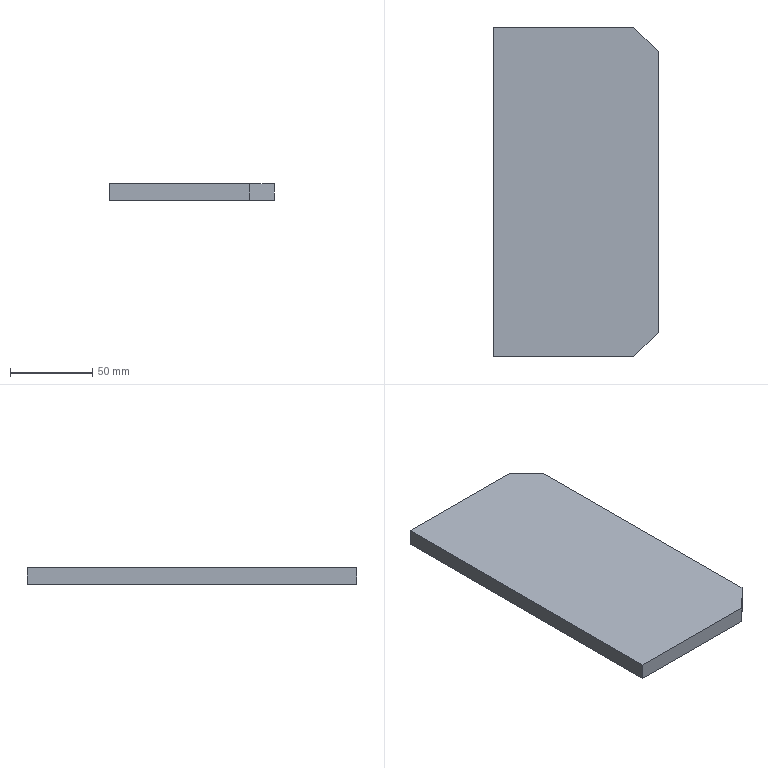Part | SolidWorks | features Chamfer 1, Extrusion 1, ICE 1 | 1 solid | 8 faces | box 100 x 200 x 10 mm | volume 197750 mm3 | plane 8
STEP:
#1=CARTESIAN_POINT('',(0.,0.,-5.));
#2=VERTEX_POINT('',#1);
#3=CARTESIAN_POINT('',(85.,0.,-5.));
#4=VERTEX_POINT('',#3);
#5=CARTESIAN_POINT('',(100.,0.,-5.));
#6=DIRECTION('',(1.,0.,0.));
#7=VECTOR('',#6,1000.);
#8=LINE('',#5,#7);
#9=EDGE_CURVE('',#2,#4,#8,.T.);
#10=ORIENTED_EDGE('',*,*,#9,.T.);
#11=CARTESIAN_POINT('',(85.,0.,5.));
#12=VERTEX_POINT('',#11);
#13=CARTESIAN_POINT('',(85.,0.,5.));
#14=DIRECTION('',(0.,0.,1.));
#15=VECTOR('',#14,1000.);
#16=LINE('',#13,#15);
#17=EDGE_CURVE('',#4,#12,#16,.T.);
#18=ORIENTED_EDGE('',*,*,#17,.T.);
#19=CARTESIAN_POINT('',(0.,0.,5.));
#20=VERTEX_POINT('',#19);
#21=CARTESIAN_POINT('',(100.,0.,5.));
#22=DIRECTION('',(1.,0.,0.));
#23=VECTOR('',#22,1000.);
#24=LINE('',#21,#23);
#25=EDGE_CURVE('',#20,#12,#24,.T.);
#26=ORIENTED_EDGE('',*,*,#25,.F.);
#27=CARTESIAN_POINT('',(0.,0.,5.));
#28=DIRECTION('',(0.,0.,-1.));
#29=VECTOR('',#28,1000.);
#30=LINE('',#27,#29);
#31=EDGE_CURVE('',#20,#2,#30,.T.);
#32=ORIENTED_EDGE('',*,*,#31,.T.);
#33=EDGE_LOOP('',(#10,#18,#26,#32));
#34=FACE_OUTER_BOUND('',#33,.T.);
#35=CARTESIAN_POINT('',(100.,0.,5.));
#36=DIRECTION('',(0.,1.,0.));
#37=DIRECTION('',(0.,0.,1.));
#38=AXIS2_PLACEMENT_3D('',#35,#36,#37);
#39=PLANE('',#38);
#40=ADVANCED_FACE('',(#34),#39,.F.);
#41=CARTESIAN_POINT('',(100.,15.,-5.));
#42=VERTEX_POINT('',#41);
#43=CARTESIAN_POINT('',(100.,185.,-5.));
#44=VERTEX_POINT('',#43);
#45=CARTESIAN_POINT('',(100.,200.,-5.));
#46=DIRECTION('',(0.,1.,0.));
#47=VECTOR('',#46,1000.);
#48=LINE('',#45,#47);
#49=EDGE_CURVE('',#42,#44,#48,.T.);
#50=ORIENTED_EDGE('',*,*,#49,.T.);
#51=CARTESIAN_POINT('',(100.,185.,5.));
#52=VERTEX_POINT('',#51);
#53=CARTESIAN_POINT('',(100.,185.,5.));
#54=DIRECTION('',(0.,0.,1.));
#55=VECTOR('',#54,1000.);
#56=LINE('',#53,#55);
#57=EDGE_CURVE('',#44,#52,#56,.T.);
#58=ORIENTED_EDGE('',*,*,#57,.T.);
#59=CARTESIAN_POINT('',(100.,15.,5.));
#60=VERTEX_POINT('',#59);
#61=CARTESIAN_POINT('',(100.,200.,5.));
#62=DIRECTION('',(0.,1.,0.));
#63=VECTOR('',#62,1000.);
#64=LINE('',#61,#63);
#65=EDGE_CURVE('',#60,#52,#64,.T.);
#66=ORIENTED_EDGE('',*,*,#65,.F.);
#67=CARTESIAN_POINT('',(100.,15.,5.));
#68=DIRECTION('',(0.,0.,-1.));
#69=VECTOR('',#68,1000.);
#70=LINE('',#67,#69);
#71=EDGE_CURVE('',#60,#42,#70,.T.);
#72=ORIENTED_EDGE('',*,*,#71,.T.);
#73=EDGE_LOOP('',(#50,#58,#66,#72));
#74=FACE_OUTER_BOUND('',#73,.T.);
#75=CARTESIAN_POINT('',(100.,200.,5.));
#76=DIRECTION('',(-1.,0.,0.));
#77=DIRECTION('',(0.,-1.,0.));
#78=AXIS2_PLACEMENT_3D('',#75,#76,#77);
#79=PLANE('',#78);
#80=ADVANCED_FACE('',(#74),#79,.F.);
#81=CARTESIAN_POINT('',(85.,200.,5.));
#82=VERTEX_POINT('',#81);
#83=CARTESIAN_POINT('',(0.,200.,5.));
#84=VERTEX_POINT('',#83);
#85=CARTESIAN_POINT('',(46.,200.,5.));
#86=DIRECTION('',(-1.,0.,0.));
#87=VECTOR('',#86,1000.);
#88=LINE('',#85,#87);
#89=EDGE_CURVE('',#82,#84,#88,.T.);
#90=ORIENTED_EDGE('',*,*,#89,.F.);
#91=CARTESIAN_POINT('',(85.,200.,-5.));
#92=VERTEX_POINT('',#91);
#93=CARTESIAN_POINT('',(85.,200.,5.));
#94=DIRECTION('',(0.,0.,-1.));
#95=VECTOR('',#94,1000.);
#96=LINE('',#93,#95);
#97=EDGE_CURVE('',#82,#92,#96,.T.);
#98=ORIENTED_EDGE('',*,*,#97,.T.);
#99=CARTESIAN_POINT('',(0.,200.,-5.));
#100=VERTEX_POINT('',#99);
#101=CARTESIAN_POINT('',(46.,200.,-5.));
#102=DIRECTION('',(-1.,0.,0.));
#103=VECTOR('',#102,1000.);
#104=LINE('',#101,#103);
#105=EDGE_CURVE('',#92,#100,#104,.T.);
#106=ORIENTED_EDGE('',*,*,#105,.T.);
#107=CARTESIAN_POINT('',(0.,200.,-72.941));
#108=DIRECTION('',(0.,0.,1.));
#109=VECTOR('',#108,1000.);
#110=LINE('',#107,#109);
#111=EDGE_CURVE('',#100,#84,#110,.T.);
#112=ORIENTED_EDGE('',*,*,#111,.T.);
#113=EDGE_LOOP('',(#90,#98,#106,#112));
#114=FACE_OUTER_BOUND('',#113,.T.);
#115=CARTESIAN_POINT('',(46.,200.,5.));
#116=DIRECTION('',(0.,-1.,0.));
#117=DIRECTION('',(0.,0.,-1.));
#118=AXIS2_PLACEMENT_3D('',#115,#116,#117);
#119=PLANE('',#118);
#120=ADVANCED_FACE('',(#114),#119,.F.);
#121=CARTESIAN_POINT('',(0.,0.,-5.));
#122=DIRECTION('',(0.,-1.,0.));
#123=VECTOR('',#122,1000.);
#124=LINE('',#121,#123);
#125=EDGE_CURVE('',#100,#2,#124,.T.);
#126=ORIENTED_EDGE('',*,*,#125,.T.);
#127=ORIENTED_EDGE('',*,*,#31,.F.);
#128=CARTESIAN_POINT('',(0.,0.,5.));
#129=DIRECTION('',(0.,-1.,0.));
#130=VECTOR('',#129,1000.);
#131=LINE('',#128,#130);
#132=EDGE_CURVE('',#84,#20,#131,.T.);
#133=ORIENTED_EDGE('',*,*,#132,.F.);
#134=ORIENTED_EDGE('',*,*,#111,.F.);
#135=EDGE_LOOP('',(#126,#127,#133,#134));
#136=FACE_OUTER_BOUND('',#135,.T.);
#137=CARTESIAN_POINT('',(0.,0.,5.));
#138=DIRECTION('',(1.,0.,0.));
#139=DIRECTION('',(0.,0.,-1.));
#140=AXIS2_PLACEMENT_3D('',#137,#138,#139);
#141=PLANE('',#140);
#142=ADVANCED_FACE('',(#136),#141,.F.);
#143=ORIENTED_EDGE('',*,*,#65,.T.);
#144=CARTESIAN_POINT('',(85.,200.,5.));
#145=DIRECTION('',(-0.7071,0.7071,0.));
#146=VECTOR('',#145,1000.);
#147=LINE('',#144,#146);
#148=EDGE_CURVE('',#52,#82,#147,.T.);
#149=ORIENTED_EDGE('',*,*,#148,.T.);
#150=ORIENTED_EDGE('',*,*,#89,.T.);
#151=ORIENTED_EDGE('',*,*,#132,.T.);
#152=ORIENTED_EDGE('',*,*,#25,.T.);
#153=CARTESIAN_POINT('',(100.,15.,5.));
#154=DIRECTION('',(0.7071,0.7071,0.));
#155=VECTOR('',#154,1000.);
#156=LINE('',#153,#155);
#157=EDGE_CURVE('',#12,#60,#156,.T.);
#158=ORIENTED_EDGE('',*,*,#157,.T.);
#159=EDGE_LOOP('',(#143,#149,#150,#151,#152,#158));
#160=FACE_OUTER_BOUND('',#159,.T.);
#161=CARTESIAN_POINT('',(0.,0.,5.));
#162=DIRECTION('',(0.,0.,-1.));
#163=DIRECTION('',(-1.,0.,0.));
#164=AXIS2_PLACEMENT_3D('',#161,#162,#163);
#165=PLANE('',#164);
#166=ADVANCED_FACE('',(#160),#165,.F.);
#167=ORIENTED_EDGE('',*,*,#105,.F.);
#168=CARTESIAN_POINT('',(142.5,142.5,-5.));
#169=DIRECTION('',(0.7071,-0.7071,0.));
#170=VECTOR('',#169,1000.);
#171=LINE('',#168,#170);
#172=EDGE_CURVE('',#92,#44,#171,.T.);
#173=ORIENTED_EDGE('',*,*,#172,.T.);
#174=ORIENTED_EDGE('',*,*,#49,.F.);
#175=CARTESIAN_POINT('',(42.5,-42.5,-5.));
#176=DIRECTION('',(-0.7071,-0.7071,0.));
#177=VECTOR('',#176,1000.);
#178=LINE('',#175,#177);
#179=EDGE_CURVE('',#42,#4,#178,.T.);
#180=ORIENTED_EDGE('',*,*,#179,.T.);
#181=ORIENTED_EDGE('',*,*,#9,.F.);
#182=ORIENTED_EDGE('',*,*,#125,.F.);
#183=EDGE_LOOP('',(#167,#173,#174,#180,#181,#182));
#184=FACE_OUTER_BOUND('',#183,.T.);
#185=CARTESIAN_POINT('',(0.,0.,-5.));
#186=DIRECTION('',(0.,0.,-1.));
#187=DIRECTION('',(-1.,0.,0.));
#188=AXIS2_PLACEMENT_3D('',#185,#186,#187);
#189=PLANE('',#188);
#190=ADVANCED_FACE('',(#184),#189,.T.);
#191=ORIENTED_EDGE('',*,*,#148,.F.);
#192=ORIENTED_EDGE('',*,*,#57,.F.);
#193=ORIENTED_EDGE('',*,*,#172,.F.);
#194=ORIENTED_EDGE('',*,*,#97,.F.);
#195=EDGE_LOOP('',(#191,#192,#193,#194));
#196=FACE_OUTER_BOUND('',#195,.T.);
#197=CARTESIAN_POINT('',(85.,200.,5.));
#198=DIRECTION('',(-0.7071,-0.7071,0.));
#199=DIRECTION('',(0.,0.,-1.));
#200=AXIS2_PLACEMENT_3D('',#197,#198,#199);
#201=PLANE('',#200);
#202=ADVANCED_FACE('',(#196),#201,.F.);
#203=ORIENTED_EDGE('',*,*,#157,.F.);
#204=ORIENTED_EDGE('',*,*,#17,.F.);
#205=ORIENTED_EDGE('',*,*,#179,.F.);
#206=ORIENTED_EDGE('',*,*,#71,.F.);
#207=EDGE_LOOP('',(#203,#204,#205,#206));
#208=FACE_OUTER_BOUND('',#207,.T.);
#209=CARTESIAN_POINT('',(100.,15.,5.));
#210=DIRECTION('',(-0.7071,0.7071,0.));
#211=DIRECTION('',(0.,0.,-1.));
#212=AXIS2_PLACEMENT_3D('',#209,#210,#211);
#213=PLANE('',#212);
#214=ADVANCED_FACE('',(#208),#213,.F.);
#215=CLOSED_SHELL('',(#40,#80,#120,#142,#166,#190,#202,#214));
#216=MANIFOLD_SOLID_BREP('',#215);
#217=CARTESIAN_POINT('',(0.,0.,0.));
#218=DIRECTION('',(0.,0.,1.));
#219=DIRECTION('',(1.,0.,0.));
#220=AXIS2_PLACEMENT_3D('',#217,#218,#219);
#221=(LENGTH_UNIT()NAMED_UNIT(*)SI_UNIT(.MILLI.,.METRE.));
#222=UNCERTAINTY_MEASURE_WITH_UNIT(LENGTH_MEASURE(0.00001),#221,'','');
#223=(NAMED_UNIT(*)PLANE_ANGLE_UNIT()SI_UNIT($,.RADIAN.));
#224=(NAMED_UNIT(*)SI_UNIT($,.STERADIAN.)SOLID_ANGLE_UNIT());
#225=(GEOMETRIC_REPRESENTATION_CONTEXT(3)GLOBAL_UNCERTAINTY_ASSIGNED_CONTEXT((#222))GLOBAL_UNIT_ASSIGNED_CONTEXT((#221,#223,#224))REPRESENTATION_CONTEXT('',''));
#226=ADVANCED_BREP_SHAPE_REPRESENTATION('',(#216,#220),#225);